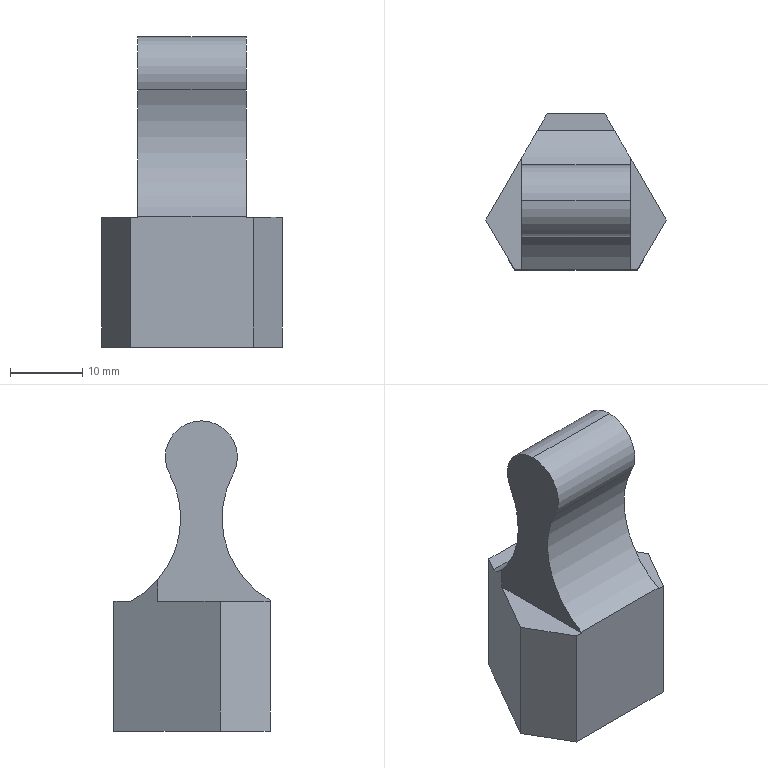Part | STEP file | Seal sleeve 7 | 1 solid | 21 faces | box 25 x 21.651 x 43 mm | volume 9390 mm3 | plane 13 | cylinder 8 | commonest cylinder face diameters 10 x4 2.5 x2 26 x2